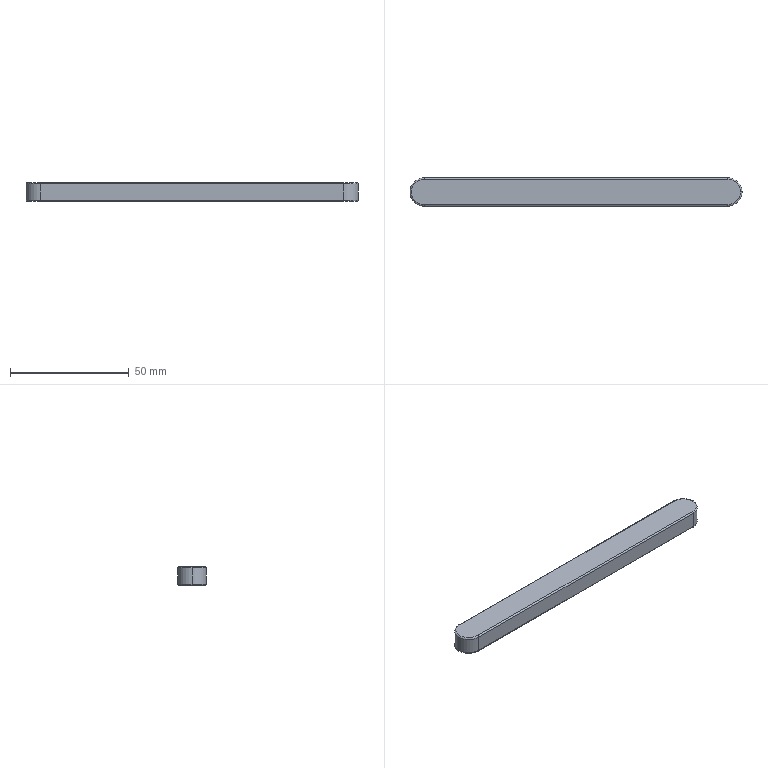Part | SolidWorks | features Extrusion 1, Fillet 1 | 1 solid | 17 faces | box 140 x 12 x 8 mm | volume 13148 mm3 | cylinder 7 | torus 6 | plane 4 | commonest cylinder face diameters 1.2 x4 12 x3
STEP:
#1=CARTESIAN_POINT('',(69.4,0.,0.));
#2=VERTEX_POINT('',#1);
#3=CARTESIAN_POINT('',(64.,-5.4,0.));
#4=VERTEX_POINT('',#3);
#5=CARTESIAN_POINT('',(64.,0.,0.));
#6=DIRECTION('',(0.,0.,-1.));
#7=DIRECTION('',(1.,0.,0.));
#8=AXIS2_PLACEMENT_3D('',#5,#6,#7);
#9=CIRCLE('',#8,5.4);
#10=EDGE_CURVE('',#2,#4,#9,.T.);
#11=ORIENTED_EDGE('',*,*,#10,.F.);
#12=CARTESIAN_POINT('',(70.,0.,0.6));
#13=VERTEX_POINT('',#12);
#14=CARTESIAN_POINT('',(69.4,0.,0.6));
#15=DIRECTION('',(0.,-1.,0.));
#16=DIRECTION('',(0.,0.,-1.));
#17=AXIS2_PLACEMENT_3D('',#14,#15,#16);
#18=CIRCLE('',#17,0.6);
#19=EDGE_CURVE('',#2,#13,#18,.T.);
#20=ORIENTED_EDGE('',*,*,#19,.T.);
#21=CARTESIAN_POINT('',(64.,-6.,0.6));
#22=VERTEX_POINT('',#21);
#23=CARTESIAN_POINT('',(64.,0.,0.6));
#24=DIRECTION('',(0.,0.,1.));
#25=DIRECTION('',(1.,0.,0.));
#26=AXIS2_PLACEMENT_3D('',#23,#24,#25);
#27=CIRCLE('',#26,6.);
#28=EDGE_CURVE('',#22,#13,#27,.T.);
#29=ORIENTED_EDGE('',*,*,#28,.F.);
#30=CARTESIAN_POINT('',(64.,-5.4,0.6));
#31=DIRECTION('',(1.,0.,0.));
#32=DIRECTION('',(0.,0.,-1.));
#33=AXIS2_PLACEMENT_3D('',#30,#31,#32);
#34=CIRCLE('',#33,0.6);
#35=EDGE_CURVE('',#22,#4,#34,.T.);
#36=ORIENTED_EDGE('',*,*,#35,.T.);
#37=EDGE_LOOP('',(#11,#20,#29,#36));
#38=FACE_OUTER_BOUND('',#37,.T.);
#39=CARTESIAN_POINT('',(64.,0.,0.6));
#40=DIRECTION('',(0.,0.,1.));
#41=DIRECTION('',(1.,0.,0.));
#42=AXIS2_PLACEMENT_3D('',#39,#40,#41);
#43=TOROIDAL_SURFACE('',#42,5.4,0.6);
#44=ADVANCED_FACE('',(#38),#43,.T.);
#45=CARTESIAN_POINT('',(70.,0.,7.4));
#46=VERTEX_POINT('',#45);
#47=CARTESIAN_POINT('',(64.,-6.,7.4));
#48=VERTEX_POINT('',#47);
#49=CARTESIAN_POINT('',(64.,0.,7.4));
#50=DIRECTION('',(0.,0.,-1.));
#51=DIRECTION('',(1.,0.,0.));
#52=AXIS2_PLACEMENT_3D('',#49,#50,#51);
#53=CIRCLE('',#52,6.);
#54=EDGE_CURVE('',#46,#48,#53,.T.);
#55=ORIENTED_EDGE('',*,*,#54,.F.);
#56=CARTESIAN_POINT('',(69.4,0.,8.));
#57=VERTEX_POINT('',#56);
#58=CARTESIAN_POINT('',(69.4,0.,7.4));
#59=DIRECTION('',(0.,-1.,0.));
#60=DIRECTION('',(0.,0.,-1.));
#61=AXIS2_PLACEMENT_3D('',#58,#59,#60);
#62=CIRCLE('',#61,0.6);
#63=EDGE_CURVE('',#46,#57,#62,.T.);
#64=ORIENTED_EDGE('',*,*,#63,.T.);
#65=CARTESIAN_POINT('',(64.,-5.4,8.));
#66=VERTEX_POINT('',#65);
#67=CARTESIAN_POINT('',(64.,0.,8.));
#68=DIRECTION('',(0.,0.,1.));
#69=DIRECTION('',(1.,0.,0.));
#70=AXIS2_PLACEMENT_3D('',#67,#68,#69);
#71=CIRCLE('',#70,5.4);
#72=EDGE_CURVE('',#66,#57,#71,.T.);
#73=ORIENTED_EDGE('',*,*,#72,.F.);
#74=CARTESIAN_POINT('',(64.,-5.4,7.4));
#75=DIRECTION('',(1.,0.,0.));
#76=DIRECTION('',(0.,0.,-1.));
#77=AXIS2_PLACEMENT_3D('',#74,#75,#76);
#78=CIRCLE('',#77,0.6);
#79=EDGE_CURVE('',#66,#48,#78,.T.);
#80=ORIENTED_EDGE('',*,*,#79,.T.);
#81=EDGE_LOOP('',(#55,#64,#73,#80));
#82=FACE_OUTER_BOUND('',#81,.T.);
#83=CARTESIAN_POINT('',(64.,0.,7.4));
#84=DIRECTION('',(0.,0.,1.));
#85=DIRECTION('',(1.,0.,0.));
#86=AXIS2_PLACEMENT_3D('',#83,#84,#85);
#87=TOROIDAL_SURFACE('',#86,5.4,0.6);
#88=ADVANCED_FACE('',(#82),#87,.T.);
#89=CARTESIAN_POINT('',(-64.,-6.,7.4));
#90=VERTEX_POINT('',#89);
#91=CARTESIAN_POINT('',(-70.,0.,7.4));
#92=VERTEX_POINT('',#91);
#93=CARTESIAN_POINT('',(-64.,0.,7.4));
#94=DIRECTION('',(0.,0.,-1.));
#95=DIRECTION('',(1.,0.,0.));
#96=AXIS2_PLACEMENT_3D('',#93,#94,#95);
#97=CIRCLE('',#96,6.);
#98=EDGE_CURVE('',#90,#92,#97,.T.);
#99=ORIENTED_EDGE('',*,*,#98,.T.);
#100=CARTESIAN_POINT('',(-70.,0.,0.6));
#101=VERTEX_POINT('',#100);
#102=CARTESIAN_POINT('',(-70.,0.,8.));
#103=DIRECTION('',(0.,0.,-1.));
#104=VECTOR('',#103,1000.);
#105=LINE('',#102,#104);
#106=EDGE_CURVE('',#92,#101,#105,.T.);
#107=ORIENTED_EDGE('',*,*,#106,.T.);
#108=CARTESIAN_POINT('',(-64.,-6.,0.6));
#109=VERTEX_POINT('',#108);
#110=CARTESIAN_POINT('',(-64.,0.,0.6));
#111=DIRECTION('',(0.,0.,1.));
#112=DIRECTION('',(1.,0.,0.));
#113=AXIS2_PLACEMENT_3D('',#110,#111,#112);
#114=CIRCLE('',#113,6.);
#115=EDGE_CURVE('',#101,#109,#114,.T.);
#116=ORIENTED_EDGE('',*,*,#115,.T.);
#117=CARTESIAN_POINT('',(-64.,-6.,8.));
#118=DIRECTION('',(0.,0.,-1.));
#119=VECTOR('',#118,1000.);
#120=LINE('',#117,#119);
#121=EDGE_CURVE('',#90,#109,#120,.T.);
#122=ORIENTED_EDGE('',*,*,#121,.F.);
#123=EDGE_LOOP('',(#99,#107,#116,#122));
#124=FACE_OUTER_BOUND('',#123,.T.);
#125=CARTESIAN_POINT('',(-64.,0.,8.));
#126=DIRECTION('',(0.,0.,-1.));
#127=DIRECTION('',(-1.,0.,0.));
#128=AXIS2_PLACEMENT_3D('',#125,#126,#127);
#129=CYLINDRICAL_SURFACE('',#128,6.);
#130=ADVANCED_FACE('',(#124),#129,.T.);
#131=ORIENTED_EDGE('',*,*,#106,.F.);
#132=CARTESIAN_POINT('',(-64.,6.,7.4));
#133=VERTEX_POINT('',#132);
#134=CARTESIAN_POINT('',(-64.,0.,7.4));
#135=DIRECTION('',(0.,0.,-1.));
#136=DIRECTION('',(1.,0.,0.));
#137=AXIS2_PLACEMENT_3D('',#134,#135,#136);
#138=CIRCLE('',#137,6.);
#139=EDGE_CURVE('',#92,#133,#138,.T.);
#140=ORIENTED_EDGE('',*,*,#139,.T.);
#141=CARTESIAN_POINT('',(-64.,6.,0.6));
#142=VERTEX_POINT('',#141);
#143=CARTESIAN_POINT('',(-64.,6.,8.));
#144=DIRECTION('',(0.,0.,-1.));
#145=VECTOR('',#144,1000.);
#146=LINE('',#143,#145);
#147=EDGE_CURVE('',#133,#142,#146,.T.);
#148=ORIENTED_EDGE('',*,*,#147,.T.);
#149=CARTESIAN_POINT('',(-64.,0.,0.6));
#150=DIRECTION('',(0.,0.,1.));
#151=DIRECTION('',(1.,0.,0.));
#152=AXIS2_PLACEMENT_3D('',#149,#150,#151);
#153=CIRCLE('',#152,6.);
#154=EDGE_CURVE('',#142,#101,#153,.T.);
#155=ORIENTED_EDGE('',*,*,#154,.T.);
#156=EDGE_LOOP('',(#131,#140,#148,#155));
#157=FACE_OUTER_BOUND('',#156,.T.);
#158=CARTESIAN_POINT('',(-64.,0.,8.));
#159=DIRECTION('',(0.,0.,-1.));
#160=DIRECTION('',(-1.,0.,0.));
#161=AXIS2_PLACEMENT_3D('',#158,#159,#160);
#162=CYLINDRICAL_SURFACE('',#161,6.);
#163=ADVANCED_FACE('',(#157),#162,.T.);
#164=CARTESIAN_POINT('',(64.,-6.,8.));
#165=DIRECTION('',(0.,0.,-1.));
#166=VECTOR('',#165,1000.);
#167=LINE('',#164,#166);
#168=EDGE_CURVE('',#48,#22,#167,.T.);
#169=ORIENTED_EDGE('',*,*,#168,.F.);
#170=CARTESIAN_POINT('',(-64.,-6.,7.4));
#171=DIRECTION('',(-1.,0.,0.));
#172=VECTOR('',#171,1000.);
#173=LINE('',#170,#172);
#174=EDGE_CURVE('',#48,#90,#173,.T.);
#175=ORIENTED_EDGE('',*,*,#174,.T.);
#176=ORIENTED_EDGE('',*,*,#121,.T.);
#177=CARTESIAN_POINT('',(-64.,-6.,0.6));
#178=DIRECTION('',(1.,0.,0.));
#179=VECTOR('',#178,1000.);
#180=LINE('',#177,#179);
#181=EDGE_CURVE('',#109,#22,#180,.T.);
#182=ORIENTED_EDGE('',*,*,#181,.T.);
#183=EDGE_LOOP('',(#169,#175,#176,#182));
#184=FACE_OUTER_BOUND('',#183,.T.);
#185=CARTESIAN_POINT('',(-64.,-6.,8.));
#186=DIRECTION('',(0.,1.,0.));
#187=DIRECTION('',(-1.,0.,0.));
#188=AXIS2_PLACEMENT_3D('',#185,#186,#187);
#189=PLANE('',#188);
#190=ADVANCED_FACE('',(#184),#189,.F.);
#191=CARTESIAN_POINT('',(64.,6.,7.4));
#192=VERTEX_POINT('',#191);
#193=CARTESIAN_POINT('',(64.,6.,0.6));
#194=VERTEX_POINT('',#193);
#195=CARTESIAN_POINT('',(64.,6.,8.));
#196=DIRECTION('',(0.,0.,-1.));
#197=VECTOR('',#196,1000.);
#198=LINE('',#195,#197);
#199=EDGE_CURVE('',#192,#194,#198,.T.);
#200=ORIENTED_EDGE('',*,*,#199,.F.);
#201=CARTESIAN_POINT('',(64.,0.,7.4));
#202=DIRECTION('',(0.,0.,-1.));
#203=DIRECTION('',(1.,0.,0.));
#204=AXIS2_PLACEMENT_3D('',#201,#202,#203);
#205=CIRCLE('',#204,6.);
#206=EDGE_CURVE('',#192,#46,#205,.T.);
#207=ORIENTED_EDGE('',*,*,#206,.T.);
#208=ORIENTED_EDGE('',*,*,#54,.T.);
#209=ORIENTED_EDGE('',*,*,#168,.T.);
#210=ORIENTED_EDGE('',*,*,#28,.T.);
#211=CARTESIAN_POINT('',(64.,0.,0.6));
#212=DIRECTION('',(0.,0.,1.));
#213=DIRECTION('',(1.,0.,0.));
#214=AXIS2_PLACEMENT_3D('',#211,#212,#213);
#215=CIRCLE('',#214,6.);
#216=EDGE_CURVE('',#13,#194,#215,.T.);
#217=ORIENTED_EDGE('',*,*,#216,.T.);
#218=EDGE_LOOP('',(#200,#207,#208,#209,#210,#217));
#219=FACE_OUTER_BOUND('',#218,.T.);
#220=CARTESIAN_POINT('',(64.,0.,8.));
#221=DIRECTION('',(0.,0.,-1.));
#222=DIRECTION('',(-1.,0.,0.));
#223=AXIS2_PLACEMENT_3D('',#220,#221,#222);
#224=CYLINDRICAL_SURFACE('',#223,6.);
#225=ADVANCED_FACE('',(#219),#224,.T.);
#226=ORIENTED_EDGE('',*,*,#147,.F.);
#227=CARTESIAN_POINT('',(64.,6.,7.4));
#228=DIRECTION('',(1.,0.,0.));
#229=VECTOR('',#228,1000.);
#230=LINE('',#227,#229);
#231=EDGE_CURVE('',#133,#192,#230,.T.);
#232=ORIENTED_EDGE('',*,*,#231,.T.);
#233=ORIENTED_EDGE('',*,*,#199,.T.);
#234=CARTESIAN_POINT('',(-64.,6.,0.6));
#235=DIRECTION('',(-1.,0.,0.));
#236=VECTOR('',#235,1000.);
#237=LINE('',#234,#236);
#238=EDGE_CURVE('',#194,#142,#237,.T.);
#239=ORIENTED_EDGE('',*,*,#238,.T.);
#240=EDGE_LOOP('',(#226,#232,#233,#239));
#241=FACE_OUTER_BOUND('',#240,.T.);
#242=CARTESIAN_POINT('',(-64.,6.,8.));
#243=DIRECTION('',(0.,-1.,0.));
#244=DIRECTION('',(1.,0.,0.));
#245=AXIS2_PLACEMENT_3D('',#242,#243,#244);
#246=PLANE('',#245);
#247=ADVANCED_FACE('',(#241),#246,.F.);
#248=CARTESIAN_POINT('',(-64.,-5.4,8.));
#249=VERTEX_POINT('',#248);
#250=CARTESIAN_POINT('',(64.,-5.4,8.));
#251=DIRECTION('',(1.,0.,0.));
#252=VECTOR('',#251,1000.);
#253=LINE('',#250,#252);
#254=EDGE_CURVE('',#249,#66,#253,.T.);
#255=ORIENTED_EDGE('',*,*,#254,.T.);
#256=ORIENTED_EDGE('',*,*,#72,.T.);
#257=CARTESIAN_POINT('',(64.,5.4,8.));
#258=VERTEX_POINT('',#257);
#259=CARTESIAN_POINT('',(64.,0.,8.));
#260=DIRECTION('',(0.,0.,1.));
#261=DIRECTION('',(1.,0.,0.));
#262=AXIS2_PLACEMENT_3D('',#259,#260,#261);
#263=CIRCLE('',#262,5.4);
#264=EDGE_CURVE('',#57,#258,#263,.T.);
#265=ORIENTED_EDGE('',*,*,#264,.T.);
#266=CARTESIAN_POINT('',(-64.,5.4,8.));
#267=VERTEX_POINT('',#266);
#268=CARTESIAN_POINT('',(-64.,5.4,8.));
#269=DIRECTION('',(-1.,0.,0.));
#270=VECTOR('',#269,1000.);
#271=LINE('',#268,#270);
#272=EDGE_CURVE('',#258,#267,#271,.T.);
#273=ORIENTED_EDGE('',*,*,#272,.T.);
#274=CARTESIAN_POINT('',(-64.,0.,8.));
#275=DIRECTION('',(0.,0.,1.));
#276=DIRECTION('',(1.,0.,0.));
#277=AXIS2_PLACEMENT_3D('',#274,#275,#276);
#278=CIRCLE('',#277,5.4);
#279=EDGE_CURVE('',#267,#249,#278,.T.);
#280=ORIENTED_EDGE('',*,*,#279,.T.);
#281=EDGE_LOOP('',(#255,#256,#265,#273,#280));
#282=FACE_OUTER_BOUND('',#281,.T.);
#283=CARTESIAN_POINT('',(-64.,0.,8.));
#284=DIRECTION('',(0.,0.,1.));
#285=DIRECTION('',(1.,0.,0.));
#286=AXIS2_PLACEMENT_3D('',#283,#284,#285);
#287=PLANE('',#286);
#288=ADVANCED_FACE('',(#282),#287,.T.);
#289=CARTESIAN_POINT('',(-64.,5.4,0.));
#290=VERTEX_POINT('',#289);
#291=CARTESIAN_POINT('',(64.,5.4,0.));
#292=VERTEX_POINT('',#291);
#293=CARTESIAN_POINT('',(-64.,5.4,0.));
#294=DIRECTION('',(1.,0.,0.));
#295=VECTOR('',#294,1000.);
#296=LINE('',#293,#295);
#297=EDGE_CURVE('',#290,#292,#296,.T.);
#298=ORIENTED_EDGE('',*,*,#297,.T.);
#299=CARTESIAN_POINT('',(64.,0.,0.));
#300=DIRECTION('',(0.,0.,-1.));
#301=DIRECTION('',(1.,0.,0.));
#302=AXIS2_PLACEMENT_3D('',#299,#300,#301);
#303=CIRCLE('',#302,5.4);
#304=EDGE_CURVE('',#292,#2,#303,.T.);
#305=ORIENTED_EDGE('',*,*,#304,.T.);
#306=ORIENTED_EDGE('',*,*,#10,.T.);
#307=CARTESIAN_POINT('',(-64.,-5.4,0.));
#308=VERTEX_POINT('',#307);
#309=CARTESIAN_POINT('',(-64.,-5.4,0.));
#310=DIRECTION('',(-1.,0.,0.));
#311=VECTOR('',#310,1000.);
#312=LINE('',#309,#311);
#313=EDGE_CURVE('',#4,#308,#312,.T.);
#314=ORIENTED_EDGE('',*,*,#313,.T.);
#315=CARTESIAN_POINT('',(-64.,0.,0.));
#316=DIRECTION('',(0.,0.,-1.));
#317=DIRECTION('',(1.,0.,0.));
#318=AXIS2_PLACEMENT_3D('',#315,#316,#317);
#319=CIRCLE('',#318,5.4);
#320=EDGE_CURVE('',#308,#290,#319,.T.);
#321=ORIENTED_EDGE('',*,*,#320,.T.);
#322=EDGE_LOOP('',(#298,#305,#306,#314,#321));
#323=FACE_OUTER_BOUND('',#322,.T.);
#324=CARTESIAN_POINT('',(-64.,0.,0.));
#325=DIRECTION('',(0.,0.,1.));
#326=DIRECTION('',(1.,0.,0.));
#327=AXIS2_PLACEMENT_3D('',#324,#325,#326);
#328=PLANE('',#327);
#329=ADVANCED_FACE('',(#323),#328,.F.);
#330=CARTESIAN_POINT('',(-64.,5.4,7.4));
#331=DIRECTION('',(1.,0.,0.));
#332=DIRECTION('',(0.,0.,-1.));
#333=AXIS2_PLACEMENT_3D('',#330,#331,#332);
#334=CIRCLE('',#333,0.6);
#335=EDGE_CURVE('',#133,#267,#334,.T.);
#336=ORIENTED_EDGE('',*,*,#335,.F.);
#337=ORIENTED_EDGE('',*,*,#139,.F.);
#338=ORIENTED_EDGE('',*,*,#98,.F.);
#339=CARTESIAN_POINT('',(-64.,-5.4,7.4));
#340=DIRECTION('',(1.,0.,0.));
#341=DIRECTION('',(0.,0.,-1.));
#342=AXIS2_PLACEMENT_3D('',#339,#340,#341);
#343=CIRCLE('',#342,0.6);
#344=EDGE_CURVE('',#249,#90,#343,.T.);
#345=ORIENTED_EDGE('',*,*,#344,.F.);
#346=ORIENTED_EDGE('',*,*,#279,.F.);
#347=EDGE_LOOP('',(#336,#337,#338,#345,#346));
#348=FACE_OUTER_BOUND('',#347,.T.);
#349=CARTESIAN_POINT('',(-64.,0.,7.4));
#350=DIRECTION('',(0.,0.,1.));
#351=DIRECTION('',(1.,0.,0.));
#352=AXIS2_PLACEMENT_3D('',#349,#350,#351);
#353=TOROIDAL_SURFACE('',#352,5.4,0.6);
#354=ADVANCED_FACE('',(#348),#353,.T.);
#355=ORIENTED_EDGE('',*,*,#344,.T.);
#356=ORIENTED_EDGE('',*,*,#174,.F.);
#357=ORIENTED_EDGE('',*,*,#79,.F.);
#358=ORIENTED_EDGE('',*,*,#254,.F.);
#359=EDGE_LOOP('',(#355,#356,#357,#358));
#360=FACE_OUTER_BOUND('',#359,.T.);
#361=CARTESIAN_POINT('',(-64.,-5.4,7.4));
#362=DIRECTION('',(-1.,0.,0.));
#363=DIRECTION('',(0.,-1.,0.));
#364=AXIS2_PLACEMENT_3D('',#361,#362,#363);
#365=CYLINDRICAL_SURFACE('',#364,0.6);
#366=ADVANCED_FACE('',(#360),#365,.T.);
#367=ORIENTED_EDGE('',*,*,#335,.T.);
#368=ORIENTED_EDGE('',*,*,#272,.F.);
#369=CARTESIAN_POINT('',(64.,5.4,7.4));
#370=DIRECTION('',(1.,0.,0.));
#371=DIRECTION('',(0.,0.,-1.));
#372=AXIS2_PLACEMENT_3D('',#369,#370,#371);
#373=CIRCLE('',#372,0.6);
#374=EDGE_CURVE('',#192,#258,#373,.T.);
#375=ORIENTED_EDGE('',*,*,#374,.F.);
#376=ORIENTED_EDGE('',*,*,#231,.F.);
#377=EDGE_LOOP('',(#367,#368,#375,#376));
#378=FACE_OUTER_BOUND('',#377,.T.);
#379=CARTESIAN_POINT('',(-64.,5.4,7.4));
#380=DIRECTION('',(1.,0.,0.));
#381=DIRECTION('',(0.,1.,0.));
#382=AXIS2_PLACEMENT_3D('',#379,#380,#381);
#383=CYLINDRICAL_SURFACE('',#382,0.6);
#384=ADVANCED_FACE('',(#378),#383,.T.);
#385=ORIENTED_EDGE('',*,*,#63,.F.);
#386=ORIENTED_EDGE('',*,*,#206,.F.);
#387=ORIENTED_EDGE('',*,*,#374,.T.);
#388=ORIENTED_EDGE('',*,*,#264,.F.);
#389=EDGE_LOOP('',(#385,#386,#387,#388));
#390=FACE_OUTER_BOUND('',#389,.T.);
#391=CARTESIAN_POINT('',(64.,0.,7.4));
#392=DIRECTION('',(0.,0.,1.));
#393=DIRECTION('',(1.,0.,0.));
#394=AXIS2_PLACEMENT_3D('',#391,#392,#393);
#395=TOROIDAL_SURFACE('',#394,5.4,0.6);
#396=ADVANCED_FACE('',(#390),#395,.T.);
#397=CARTESIAN_POINT('',(-64.,5.4,0.6));
#398=DIRECTION('',(1.,0.,0.));
#399=DIRECTION('',(0.,0.,-1.));
#400=AXIS2_PLACEMENT_3D('',#397,#398,#399);
#401=CIRCLE('',#400,0.6);
#402=EDGE_CURVE('',#290,#142,#401,.T.);
#403=ORIENTED_EDGE('',*,*,#402,.F.);
#404=ORIENTED_EDGE('',*,*,#320,.F.);
#405=CARTESIAN_POINT('',(-64.,-5.4,0.6));
#406=DIRECTION('',(1.,0.,0.));
#407=DIRECTION('',(0.,0.,-1.));
#408=AXIS2_PLACEMENT_3D('',#405,#406,#407);
#409=CIRCLE('',#408,0.6);
#410=EDGE_CURVE('',#109,#308,#409,.T.);
#411=ORIENTED_EDGE('',*,*,#410,.F.);
#412=ORIENTED_EDGE('',*,*,#115,.F.);
#413=ORIENTED_EDGE('',*,*,#154,.F.);
#414=EDGE_LOOP('',(#403,#404,#411,#412,#413));
#415=FACE_OUTER_BOUND('',#414,.T.);
#416=CARTESIAN_POINT('',(-64.,0.,0.6));
#417=DIRECTION('',(0.,0.,1.));
#418=DIRECTION('',(1.,0.,0.));
#419=AXIS2_PLACEMENT_3D('',#416,#417,#418);
#420=TOROIDAL_SURFACE('',#419,5.4,0.6);
#421=ADVANCED_FACE('',(#415),#420,.T.);
#422=ORIENTED_EDGE('',*,*,#410,.T.);
#423=ORIENTED_EDGE('',*,*,#313,.F.);
#424=ORIENTED_EDGE('',*,*,#35,.F.);
#425=ORIENTED_EDGE('',*,*,#181,.F.);
#426=EDGE_LOOP('',(#422,#423,#424,#425));
#427=FACE_OUTER_BOUND('',#426,.T.);
#428=CARTESIAN_POINT('',(-64.,-5.4,0.6));
#429=DIRECTION('',(1.,0.,0.));
#430=DIRECTION('',(0.,1.,0.));
#431=AXIS2_PLACEMENT_3D('',#428,#429,#430);
#432=CYLINDRICAL_SURFACE('',#431,0.6);
#433=ADVANCED_FACE('',(#427),#432,.T.);
#434=ORIENTED_EDGE('',*,*,#402,.T.);
#435=ORIENTED_EDGE('',*,*,#238,.F.);
#436=CARTESIAN_POINT('',(64.,5.4,0.6));
#437=DIRECTION('',(1.,0.,0.));
#438=DIRECTION('',(0.,0.,-1.));
#439=AXIS2_PLACEMENT_3D('',#436,#437,#438);
#440=CIRCLE('',#439,0.6);
#441=EDGE_CURVE('',#292,#194,#440,.T.);
#442=ORIENTED_EDGE('',*,*,#441,.F.);
#443=ORIENTED_EDGE('',*,*,#297,.F.);
#444=EDGE_LOOP('',(#434,#435,#442,#443));
#445=FACE_OUTER_BOUND('',#444,.T.);
#446=CARTESIAN_POINT('',(-64.,5.4,0.6));
#447=DIRECTION('',(-1.,0.,0.));
#448=DIRECTION('',(0.,-1.,0.));
#449=AXIS2_PLACEMENT_3D('',#446,#447,#448);
#450=CYLINDRICAL_SURFACE('',#449,0.6);
#451=ADVANCED_FACE('',(#445),#450,.T.);
#452=ORIENTED_EDGE('',*,*,#19,.F.);
#453=ORIENTED_EDGE('',*,*,#304,.F.);
#454=ORIENTED_EDGE('',*,*,#441,.T.);
#455=ORIENTED_EDGE('',*,*,#216,.F.);
#456=EDGE_LOOP('',(#452,#453,#454,#455));
#457=FACE_OUTER_BOUND('',#456,.T.);
#458=CARTESIAN_POINT('',(64.,0.,0.6));
#459=DIRECTION('',(0.,0.,1.));
#460=DIRECTION('',(1.,0.,0.));
#461=AXIS2_PLACEMENT_3D('',#458,#459,#460);
#462=TOROIDAL_SURFACE('',#461,5.4,0.6);
#463=ADVANCED_FACE('',(#457),#462,.T.);
#464=CLOSED_SHELL('',(#44,#88,#130,#163,#190,#225,#247,#288,#329,#354,#366,#384,#396,#421,#433,#451,#463));
#465=MANIFOLD_SOLID_BREP('',#464);
#466=CARTESIAN_POINT('',(0.,0.,0.));
#467=DIRECTION('',(0.,0.,1.));
#468=DIRECTION('',(1.,0.,0.));
#469=AXIS2_PLACEMENT_3D('',#466,#467,#468);
#470=(LENGTH_UNIT()NAMED_UNIT(*)SI_UNIT(.MILLI.,.METRE.));
#471=UNCERTAINTY_MEASURE_WITH_UNIT(LENGTH_MEASURE(0.00001),#470,'','');
#472=(NAMED_UNIT(*)PLANE_ANGLE_UNIT()SI_UNIT($,.RADIAN.));
#473=(NAMED_UNIT(*)SI_UNIT($,.STERADIAN.)SOLID_ANGLE_UNIT());
#474=(GEOMETRIC_REPRESENTATION_CONTEXT(3)GLOBAL_UNCERTAINTY_ASSIGNED_CONTEXT((#471))GLOBAL_UNIT_ASSIGNED_CONTEXT((#470,#472,#473))REPRESENTATION_CONTEXT('',''));
#475=ADVANCED_BREP_SHAPE_REPRESENTATION('',(#465,#469),#474);